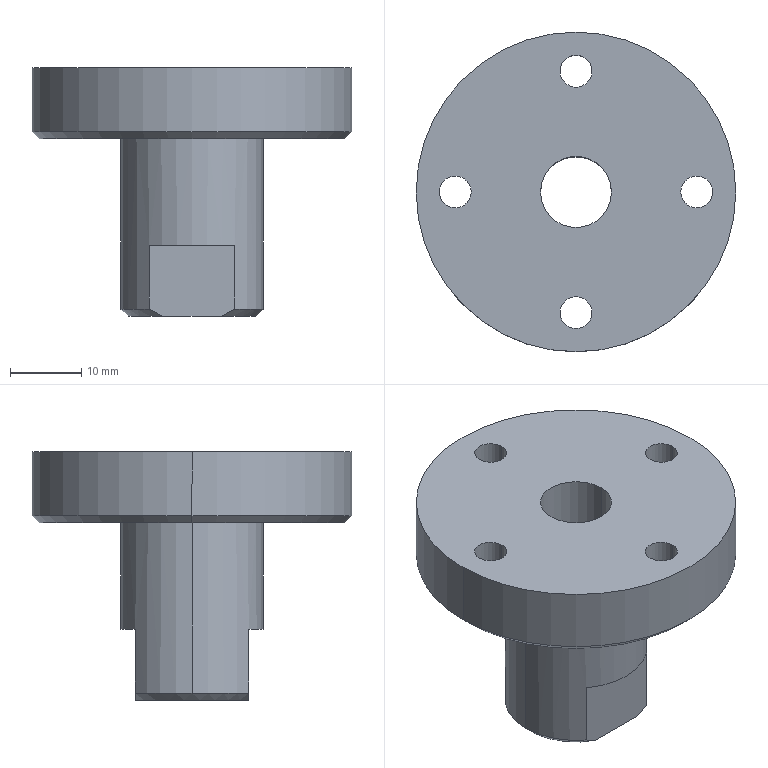Part | STEP file | Connector | 1 solid | 38 faces | box 45 x 45 x 35 mm | volume 19325 mm3 | cylinder 22 | plane 11 | cone 5 | commonest cylinder face diameters 4.5 x8 8 x8 10 x2 20 x2 45 x2